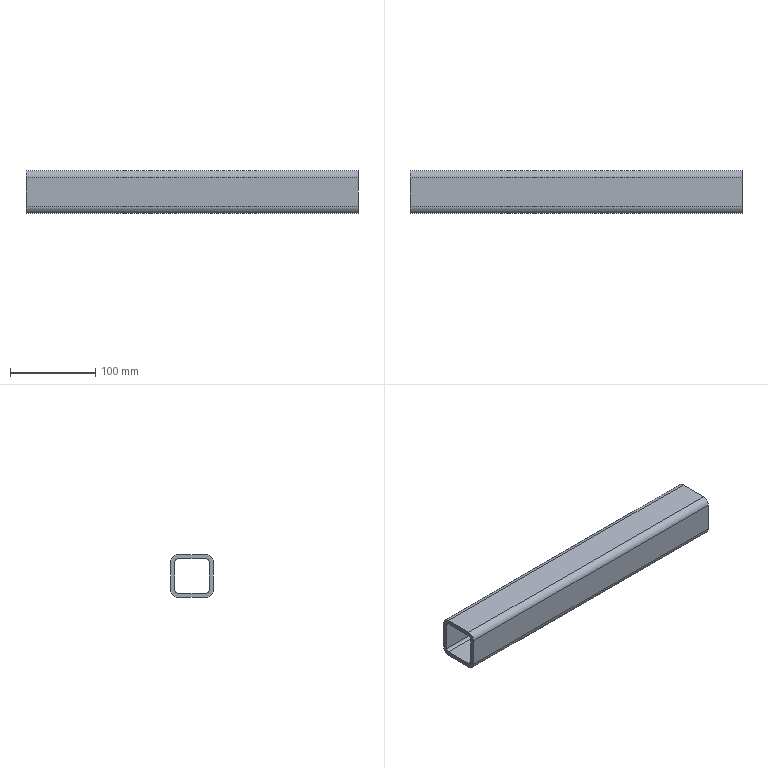Part | SolidWorks | features WeldMemberFeat 1, WeldmentFeature 1 | 1 solid | 18 faces | box 390 x 50 x 50 mm | volume 332587 mm3 | plane 10 | cylinder 8 | commonest cylinder face diameters 6 x4 16 x4
STEP:
#1=CARTESIAN_POINT('',(-88.434,25.,17.));
#2=VERTEX_POINT('',#1);
#3=CARTESIAN_POINT('',(-88.434,17.,25.));
#4=VERTEX_POINT('',#3);
#5=CARTESIAN_POINT('',(-88.434,17.,17.));
#6=DIRECTION('',(1.,0.,0.));
#7=DIRECTION('',(0.,0.,-1.));
#8=AXIS2_PLACEMENT_3D('',#5,#6,#7);
#9=CIRCLE('',#8,8.);
#10=EDGE_CURVE('',#2,#4,#9,.T.);
#11=ORIENTED_EDGE('',*,*,#10,.T.);
#12=CARTESIAN_POINT('',(301.566,17.,25.));
#13=VERTEX_POINT('',#12);
#14=CARTESIAN_POINT('',(301.566,17.,25.));
#15=DIRECTION('',(-1.,0.,0.));
#16=VECTOR('',#15,1000.);
#17=LINE('',#14,#16);
#18=EDGE_CURVE('',#13,#4,#17,.T.);
#19=ORIENTED_EDGE('',*,*,#18,.F.);
#20=CARTESIAN_POINT('',(301.566,25.,17.));
#21=VERTEX_POINT('',#20);
#22=CARTESIAN_POINT('',(301.566,17.,17.));
#23=DIRECTION('',(1.,0.,0.));
#24=DIRECTION('',(0.,0.,-1.));
#25=AXIS2_PLACEMENT_3D('',#22,#23,#24);
#26=CIRCLE('',#25,8.);
#27=EDGE_CURVE('',#21,#13,#26,.T.);
#28=ORIENTED_EDGE('',*,*,#27,.F.);
#29=CARTESIAN_POINT('',(301.566,25.,17.));
#30=DIRECTION('',(-1.,0.,0.));
#31=VECTOR('',#30,1000.);
#32=LINE('',#29,#31);
#33=EDGE_CURVE('',#21,#2,#32,.T.);
#34=ORIENTED_EDGE('',*,*,#33,.T.);
#35=EDGE_LOOP('',(#11,#19,#28,#34));
#36=FACE_OUTER_BOUND('',#35,.T.);
#37=CARTESIAN_POINT('',(301.566,17.,17.));
#38=DIRECTION('',(-1.,0.,0.));
#39=DIRECTION('',(0.,0.,1.));
#40=AXIS2_PLACEMENT_3D('',#37,#38,#39);
#41=CYLINDRICAL_SURFACE('',#40,8.);
#42=ADVANCED_FACE('',(#36),#41,.T.);
#43=CARTESIAN_POINT('',(-88.434,-17.,25.));
#44=VERTEX_POINT('',#43);
#45=CARTESIAN_POINT('',(-88.434,17.,25.));
#46=DIRECTION('',(0.,-1.,0.));
#47=VECTOR('',#46,1000.);
#48=LINE('',#45,#47);
#49=EDGE_CURVE('',#4,#44,#48,.T.);
#50=ORIENTED_EDGE('',*,*,#49,.T.);
#51=CARTESIAN_POINT('',(301.566,-17.,25.));
#52=VERTEX_POINT('',#51);
#53=CARTESIAN_POINT('',(301.566,-17.,25.));
#54=DIRECTION('',(-1.,0.,0.));
#55=VECTOR('',#54,1000.);
#56=LINE('',#53,#55);
#57=EDGE_CURVE('',#52,#44,#56,.T.);
#58=ORIENTED_EDGE('',*,*,#57,.F.);
#59=CARTESIAN_POINT('',(301.566,17.,25.));
#60=DIRECTION('',(0.,-1.,0.));
#61=VECTOR('',#60,1000.);
#62=LINE('',#59,#61);
#63=EDGE_CURVE('',#13,#52,#62,.T.);
#64=ORIENTED_EDGE('',*,*,#63,.F.);
#65=ORIENTED_EDGE('',*,*,#18,.T.);
#66=EDGE_LOOP('',(#50,#58,#64,#65));
#67=FACE_OUTER_BOUND('',#66,.T.);
#68=CARTESIAN_POINT('',(301.566,17.,25.));
#69=DIRECTION('',(0.,0.,-1.));
#70=DIRECTION('',(-1.,0.,0.));
#71=AXIS2_PLACEMENT_3D('',#68,#69,#70);
#72=PLANE('',#71);
#73=ADVANCED_FACE('',(#67),#72,.F.);
#74=CARTESIAN_POINT('',(-88.434,-25.,17.));
#75=VERTEX_POINT('',#74);
#76=CARTESIAN_POINT('',(-88.434,-17.,17.));
#77=DIRECTION('',(1.,0.,0.));
#78=DIRECTION('',(0.,0.,-1.));
#79=AXIS2_PLACEMENT_3D('',#76,#77,#78);
#80=CIRCLE('',#79,8.);
#81=EDGE_CURVE('',#44,#75,#80,.T.);
#82=ORIENTED_EDGE('',*,*,#81,.T.);
#83=CARTESIAN_POINT('',(301.566,-25.,17.));
#84=VERTEX_POINT('',#83);
#85=CARTESIAN_POINT('',(301.566,-25.,17.));
#86=DIRECTION('',(-1.,0.,0.));
#87=VECTOR('',#86,1000.);
#88=LINE('',#85,#87);
#89=EDGE_CURVE('',#84,#75,#88,.T.);
#90=ORIENTED_EDGE('',*,*,#89,.F.);
#91=CARTESIAN_POINT('',(301.566,-17.,17.));
#92=DIRECTION('',(1.,0.,0.));
#93=DIRECTION('',(0.,0.,-1.));
#94=AXIS2_PLACEMENT_3D('',#91,#92,#93);
#95=CIRCLE('',#94,8.);
#96=EDGE_CURVE('',#52,#84,#95,.T.);
#97=ORIENTED_EDGE('',*,*,#96,.F.);
#98=ORIENTED_EDGE('',*,*,#57,.T.);
#99=EDGE_LOOP('',(#82,#90,#97,#98));
#100=FACE_OUTER_BOUND('',#99,.T.);
#101=CARTESIAN_POINT('',(301.566,-17.,17.));
#102=DIRECTION('',(-1.,0.,0.));
#103=DIRECTION('',(0.,0.,1.));
#104=AXIS2_PLACEMENT_3D('',#101,#102,#103);
#105=CYLINDRICAL_SURFACE('',#104,8.);
#106=ADVANCED_FACE('',(#100),#105,.T.);
#107=CARTESIAN_POINT('',(-88.434,-25.,-17.));
#108=VERTEX_POINT('',#107);
#109=CARTESIAN_POINT('',(-88.434,-25.,-17.));
#110=DIRECTION('',(0.,0.,-1.));
#111=VECTOR('',#110,1000.);
#112=LINE('',#109,#111);
#113=EDGE_CURVE('',#75,#108,#112,.T.);
#114=ORIENTED_EDGE('',*,*,#113,.T.);
#115=CARTESIAN_POINT('',(301.566,-25.,-17.));
#116=VERTEX_POINT('',#115);
#117=CARTESIAN_POINT('',(301.566,-25.,-17.));
#118=DIRECTION('',(-1.,0.,0.));
#119=VECTOR('',#118,1000.);
#120=LINE('',#117,#119);
#121=EDGE_CURVE('',#116,#108,#120,.T.);
#122=ORIENTED_EDGE('',*,*,#121,.F.);
#123=CARTESIAN_POINT('',(301.566,-25.,-17.));
#124=DIRECTION('',(0.,0.,-1.));
#125=VECTOR('',#124,1000.);
#126=LINE('',#123,#125);
#127=EDGE_CURVE('',#84,#116,#126,.T.);
#128=ORIENTED_EDGE('',*,*,#127,.F.);
#129=ORIENTED_EDGE('',*,*,#89,.T.);
#130=EDGE_LOOP('',(#114,#122,#128,#129));
#131=FACE_OUTER_BOUND('',#130,.T.);
#132=CARTESIAN_POINT('',(301.566,-25.,-17.));
#133=DIRECTION('',(0.,1.,0.));
#134=DIRECTION('',(0.,0.,1.));
#135=AXIS2_PLACEMENT_3D('',#132,#133,#134);
#136=PLANE('',#135);
#137=ADVANCED_FACE('',(#131),#136,.F.);
#138=CARTESIAN_POINT('',(-88.434,-17.,-25.));
#139=VERTEX_POINT('',#138);
#140=CARTESIAN_POINT('',(-88.434,-17.,-17.));
#141=DIRECTION('',(1.,0.,0.));
#142=DIRECTION('',(0.,0.,-1.));
#143=AXIS2_PLACEMENT_3D('',#140,#141,#142);
#144=CIRCLE('',#143,8.);
#145=EDGE_CURVE('',#108,#139,#144,.T.);
#146=ORIENTED_EDGE('',*,*,#145,.T.);
#147=CARTESIAN_POINT('',(301.566,-17.,-25.));
#148=VERTEX_POINT('',#147);
#149=CARTESIAN_POINT('',(301.566,-17.,-25.));
#150=DIRECTION('',(-1.,0.,0.));
#151=VECTOR('',#150,1000.);
#152=LINE('',#149,#151);
#153=EDGE_CURVE('',#148,#139,#152,.T.);
#154=ORIENTED_EDGE('',*,*,#153,.F.);
#155=CARTESIAN_POINT('',(301.566,-17.,-17.));
#156=DIRECTION('',(1.,0.,0.));
#157=DIRECTION('',(0.,0.,-1.));
#158=AXIS2_PLACEMENT_3D('',#155,#156,#157);
#159=CIRCLE('',#158,8.);
#160=EDGE_CURVE('',#116,#148,#159,.T.);
#161=ORIENTED_EDGE('',*,*,#160,.F.);
#162=ORIENTED_EDGE('',*,*,#121,.T.);
#163=EDGE_LOOP('',(#146,#154,#161,#162));
#164=FACE_OUTER_BOUND('',#163,.T.);
#165=CARTESIAN_POINT('',(301.566,-17.,-17.));
#166=DIRECTION('',(-1.,0.,0.));
#167=DIRECTION('',(0.,0.,1.));
#168=AXIS2_PLACEMENT_3D('',#165,#166,#167);
#169=CYLINDRICAL_SURFACE('',#168,8.);
#170=ADVANCED_FACE('',(#164),#169,.T.);
#171=CARTESIAN_POINT('',(-88.434,17.,-25.));
#172=VERTEX_POINT('',#171);
#173=CARTESIAN_POINT('',(-88.434,-17.,-25.));
#174=DIRECTION('',(0.,1.,0.));
#175=VECTOR('',#174,1000.);
#176=LINE('',#173,#175);
#177=EDGE_CURVE('',#139,#172,#176,.T.);
#178=ORIENTED_EDGE('',*,*,#177,.T.);
#179=CARTESIAN_POINT('',(301.566,17.,-25.));
#180=VERTEX_POINT('',#179);
#181=CARTESIAN_POINT('',(301.566,17.,-25.));
#182=DIRECTION('',(-1.,0.,0.));
#183=VECTOR('',#182,1000.);
#184=LINE('',#181,#183);
#185=EDGE_CURVE('',#180,#172,#184,.T.);
#186=ORIENTED_EDGE('',*,*,#185,.F.);
#187=CARTESIAN_POINT('',(301.566,-17.,-25.));
#188=DIRECTION('',(0.,1.,0.));
#189=VECTOR('',#188,1000.);
#190=LINE('',#187,#189);
#191=EDGE_CURVE('',#148,#180,#190,.T.);
#192=ORIENTED_EDGE('',*,*,#191,.F.);
#193=ORIENTED_EDGE('',*,*,#153,.T.);
#194=EDGE_LOOP('',(#178,#186,#192,#193));
#195=FACE_OUTER_BOUND('',#194,.T.);
#196=CARTESIAN_POINT('',(301.566,-17.,-25.));
#197=DIRECTION('',(0.,0.,1.));
#198=DIRECTION('',(1.,0.,0.));
#199=AXIS2_PLACEMENT_3D('',#196,#197,#198);
#200=PLANE('',#199);
#201=ADVANCED_FACE('',(#195),#200,.F.);
#202=CARTESIAN_POINT('',(-88.434,25.,-17.));
#203=VERTEX_POINT('',#202);
#204=CARTESIAN_POINT('',(-88.434,17.,-17.));
#205=DIRECTION('',(1.,0.,0.));
#206=DIRECTION('',(0.,0.,-1.));
#207=AXIS2_PLACEMENT_3D('',#204,#205,#206);
#208=CIRCLE('',#207,8.);
#209=EDGE_CURVE('',#172,#203,#208,.T.);
#210=ORIENTED_EDGE('',*,*,#209,.T.);
#211=CARTESIAN_POINT('',(301.566,25.,-17.));
#212=VERTEX_POINT('',#211);
#213=CARTESIAN_POINT('',(301.566,25.,-17.));
#214=DIRECTION('',(-1.,0.,0.));
#215=VECTOR('',#214,1000.);
#216=LINE('',#213,#215);
#217=EDGE_CURVE('',#212,#203,#216,.T.);
#218=ORIENTED_EDGE('',*,*,#217,.F.);
#219=CARTESIAN_POINT('',(301.566,17.,-17.));
#220=DIRECTION('',(1.,0.,0.));
#221=DIRECTION('',(0.,0.,-1.));
#222=AXIS2_PLACEMENT_3D('',#219,#220,#221);
#223=CIRCLE('',#222,8.);
#224=EDGE_CURVE('',#180,#212,#223,.T.);
#225=ORIENTED_EDGE('',*,*,#224,.F.);
#226=ORIENTED_EDGE('',*,*,#185,.T.);
#227=EDGE_LOOP('',(#210,#218,#225,#226));
#228=FACE_OUTER_BOUND('',#227,.T.);
#229=CARTESIAN_POINT('',(301.566,17.,-17.));
#230=DIRECTION('',(-1.,0.,0.));
#231=DIRECTION('',(0.,0.,1.));
#232=AXIS2_PLACEMENT_3D('',#229,#230,#231);
#233=CYLINDRICAL_SURFACE('',#232,8.);
#234=ADVANCED_FACE('',(#228),#233,.T.);
#235=CARTESIAN_POINT('',(-88.434,-17.,20.));
#236=VERTEX_POINT('',#235);
#237=CARTESIAN_POINT('',(-88.434,-20.,17.));
#238=VERTEX_POINT('',#237);
#239=CARTESIAN_POINT('',(-88.434,-17.,17.));
#240=DIRECTION('',(1.,0.,0.));
#241=DIRECTION('',(0.,0.,-1.));
#242=AXIS2_PLACEMENT_3D('',#239,#240,#241);
#243=CIRCLE('',#242,3.);
#244=EDGE_CURVE('',#236,#238,#243,.T.);
#245=ORIENTED_EDGE('',*,*,#244,.F.);
#246=CARTESIAN_POINT('',(301.566,-17.,20.));
#247=VERTEX_POINT('',#246);
#248=CARTESIAN_POINT('',(301.566,-17.,20.));
#249=DIRECTION('',(-1.,0.,0.));
#250=VECTOR('',#249,1000.);
#251=LINE('',#248,#250);
#252=EDGE_CURVE('',#247,#236,#251,.T.);
#253=ORIENTED_EDGE('',*,*,#252,.F.);
#254=CARTESIAN_POINT('',(301.566,-20.,17.));
#255=VERTEX_POINT('',#254);
#256=CARTESIAN_POINT('',(301.566,-17.,17.));
#257=DIRECTION('',(1.,0.,0.));
#258=DIRECTION('',(0.,0.,-1.));
#259=AXIS2_PLACEMENT_3D('',#256,#257,#258);
#260=CIRCLE('',#259,3.);
#261=EDGE_CURVE('',#247,#255,#260,.T.);
#262=ORIENTED_EDGE('',*,*,#261,.T.);
#263=CARTESIAN_POINT('',(301.566,-20.,17.));
#264=DIRECTION('',(-1.,0.,0.));
#265=VECTOR('',#264,1000.);
#266=LINE('',#263,#265);
#267=EDGE_CURVE('',#255,#238,#266,.T.);
#268=ORIENTED_EDGE('',*,*,#267,.T.);
#269=EDGE_LOOP('',(#245,#253,#262,#268));
#270=FACE_OUTER_BOUND('',#269,.T.);
#271=CARTESIAN_POINT('',(301.566,-17.,17.));
#272=DIRECTION('',(-1.,0.,0.));
#273=DIRECTION('',(0.,0.,1.));
#274=AXIS2_PLACEMENT_3D('',#271,#272,#273);
#275=CYLINDRICAL_SURFACE('',#274,3.);
#276=ADVANCED_FACE('',(#270),#275,.F.);
#277=CARTESIAN_POINT('',(-88.434,17.,20.));
#278=VERTEX_POINT('',#277);
#279=CARTESIAN_POINT('',(-88.434,17.,20.));
#280=DIRECTION('',(0.,-1.,0.));
#281=VECTOR('',#280,1000.);
#282=LINE('',#279,#281);
#283=EDGE_CURVE('',#278,#236,#282,.T.);
#284=ORIENTED_EDGE('',*,*,#283,.F.);
#285=CARTESIAN_POINT('',(301.566,17.,20.));
#286=VERTEX_POINT('',#285);
#287=CARTESIAN_POINT('',(301.566,17.,20.));
#288=DIRECTION('',(-1.,0.,0.));
#289=VECTOR('',#288,1000.);
#290=LINE('',#287,#289);
#291=EDGE_CURVE('',#286,#278,#290,.T.);
#292=ORIENTED_EDGE('',*,*,#291,.F.);
#293=CARTESIAN_POINT('',(301.566,17.,20.));
#294=DIRECTION('',(0.,-1.,0.));
#295=VECTOR('',#294,1000.);
#296=LINE('',#293,#295);
#297=EDGE_CURVE('',#286,#247,#296,.T.);
#298=ORIENTED_EDGE('',*,*,#297,.T.);
#299=ORIENTED_EDGE('',*,*,#252,.T.);
#300=EDGE_LOOP('',(#284,#292,#298,#299));
#301=FACE_OUTER_BOUND('',#300,.T.);
#302=CARTESIAN_POINT('',(301.566,17.,20.));
#303=DIRECTION('',(0.,0.,-1.));
#304=DIRECTION('',(-1.,0.,0.));
#305=AXIS2_PLACEMENT_3D('',#302,#303,#304);
#306=PLANE('',#305);
#307=ADVANCED_FACE('',(#301),#306,.T.);
#308=CARTESIAN_POINT('',(-88.434,20.,17.));
#309=VERTEX_POINT('',#308);
#310=CARTESIAN_POINT('',(-88.434,17.,17.));
#311=DIRECTION('',(1.,0.,0.));
#312=DIRECTION('',(0.,0.,-1.));
#313=AXIS2_PLACEMENT_3D('',#310,#311,#312);
#314=CIRCLE('',#313,3.);
#315=EDGE_CURVE('',#309,#278,#314,.T.);
#316=ORIENTED_EDGE('',*,*,#315,.F.);
#317=CARTESIAN_POINT('',(301.566,20.,17.));
#318=VERTEX_POINT('',#317);
#319=CARTESIAN_POINT('',(301.566,20.,17.));
#320=DIRECTION('',(-1.,0.,0.));
#321=VECTOR('',#320,1000.);
#322=LINE('',#319,#321);
#323=EDGE_CURVE('',#318,#309,#322,.T.);
#324=ORIENTED_EDGE('',*,*,#323,.F.);
#325=CARTESIAN_POINT('',(301.566,17.,17.));
#326=DIRECTION('',(1.,0.,0.));
#327=DIRECTION('',(0.,0.,-1.));
#328=AXIS2_PLACEMENT_3D('',#325,#326,#327);
#329=CIRCLE('',#328,3.);
#330=EDGE_CURVE('',#318,#286,#329,.T.);
#331=ORIENTED_EDGE('',*,*,#330,.T.);
#332=ORIENTED_EDGE('',*,*,#291,.T.);
#333=EDGE_LOOP('',(#316,#324,#331,#332));
#334=FACE_OUTER_BOUND('',#333,.T.);
#335=CARTESIAN_POINT('',(301.566,17.,17.));
#336=DIRECTION('',(-1.,0.,0.));
#337=DIRECTION('',(0.,0.,1.));
#338=AXIS2_PLACEMENT_3D('',#335,#336,#337);
#339=CYLINDRICAL_SURFACE('',#338,3.);
#340=ADVANCED_FACE('',(#334),#339,.F.);
#341=CARTESIAN_POINT('',(-88.434,20.,-17.));
#342=VERTEX_POINT('',#341);
#343=CARTESIAN_POINT('',(-88.434,20.,17.));
#344=DIRECTION('',(0.,0.,1.));
#345=VECTOR('',#344,1000.);
#346=LINE('',#343,#345);
#347=EDGE_CURVE('',#342,#309,#346,.T.);
#348=ORIENTED_EDGE('',*,*,#347,.F.);
#349=CARTESIAN_POINT('',(301.566,20.,-17.));
#350=VERTEX_POINT('',#349);
#351=CARTESIAN_POINT('',(301.566,20.,-17.));
#352=DIRECTION('',(-1.,0.,0.));
#353=VECTOR('',#352,1000.);
#354=LINE('',#351,#353);
#355=EDGE_CURVE('',#350,#342,#354,.T.);
#356=ORIENTED_EDGE('',*,*,#355,.F.);
#357=CARTESIAN_POINT('',(301.566,20.,17.));
#358=DIRECTION('',(0.,0.,1.));
#359=VECTOR('',#358,1000.);
#360=LINE('',#357,#359);
#361=EDGE_CURVE('',#350,#318,#360,.T.);
#362=ORIENTED_EDGE('',*,*,#361,.T.);
#363=ORIENTED_EDGE('',*,*,#323,.T.);
#364=EDGE_LOOP('',(#348,#356,#362,#363));
#365=FACE_OUTER_BOUND('',#364,.T.);
#366=CARTESIAN_POINT('',(301.566,20.,17.));
#367=DIRECTION('',(0.,-1.,0.));
#368=DIRECTION('',(0.,0.,-1.));
#369=AXIS2_PLACEMENT_3D('',#366,#367,#368);
#370=PLANE('',#369);
#371=ADVANCED_FACE('',(#365),#370,.T.);
#372=CARTESIAN_POINT('',(-88.434,17.,-20.));
#373=VERTEX_POINT('',#372);
#374=CARTESIAN_POINT('',(-88.434,17.,-17.));
#375=DIRECTION('',(1.,0.,0.));
#376=DIRECTION('',(0.,0.,-1.));
#377=AXIS2_PLACEMENT_3D('',#374,#375,#376);
#378=CIRCLE('',#377,3.);
#379=EDGE_CURVE('',#373,#342,#378,.T.);
#380=ORIENTED_EDGE('',*,*,#379,.F.);
#381=CARTESIAN_POINT('',(301.566,17.,-20.));
#382=VERTEX_POINT('',#381);
#383=CARTESIAN_POINT('',(301.566,17.,-20.));
#384=DIRECTION('',(-1.,0.,0.));
#385=VECTOR('',#384,1000.);
#386=LINE('',#383,#385);
#387=EDGE_CURVE('',#382,#373,#386,.T.);
#388=ORIENTED_EDGE('',*,*,#387,.F.);
#389=CARTESIAN_POINT('',(301.566,17.,-17.));
#390=DIRECTION('',(1.,0.,0.));
#391=DIRECTION('',(0.,0.,-1.));
#392=AXIS2_PLACEMENT_3D('',#389,#390,#391);
#393=CIRCLE('',#392,3.);
#394=EDGE_CURVE('',#382,#350,#393,.T.);
#395=ORIENTED_EDGE('',*,*,#394,.T.);
#396=ORIENTED_EDGE('',*,*,#355,.T.);
#397=EDGE_LOOP('',(#380,#388,#395,#396));
#398=FACE_OUTER_BOUND('',#397,.T.);
#399=CARTESIAN_POINT('',(301.566,17.,-17.));
#400=DIRECTION('',(-1.,0.,0.));
#401=DIRECTION('',(0.,0.,1.));
#402=AXIS2_PLACEMENT_3D('',#399,#400,#401);
#403=CYLINDRICAL_SURFACE('',#402,3.);
#404=ADVANCED_FACE('',(#398),#403,.F.);
#405=CARTESIAN_POINT('',(-88.434,-17.,-20.));
#406=VERTEX_POINT('',#405);
#407=CARTESIAN_POINT('',(-88.434,-17.,-20.));
#408=DIRECTION('',(0.,1.,0.));
#409=VECTOR('',#408,1000.);
#410=LINE('',#407,#409);
#411=EDGE_CURVE('',#406,#373,#410,.T.);
#412=ORIENTED_EDGE('',*,*,#411,.F.);
#413=CARTESIAN_POINT('',(301.566,-17.,-20.));
#414=VERTEX_POINT('',#413);
#415=CARTESIAN_POINT('',(301.566,-17.,-20.));
#416=DIRECTION('',(-1.,0.,0.));
#417=VECTOR('',#416,1000.);
#418=LINE('',#415,#417);
#419=EDGE_CURVE('',#414,#406,#418,.T.);
#420=ORIENTED_EDGE('',*,*,#419,.F.);
#421=CARTESIAN_POINT('',(301.566,-17.,-20.));
#422=DIRECTION('',(0.,1.,0.));
#423=VECTOR('',#422,1000.);
#424=LINE('',#421,#423);
#425=EDGE_CURVE('',#414,#382,#424,.T.);
#426=ORIENTED_EDGE('',*,*,#425,.T.);
#427=ORIENTED_EDGE('',*,*,#387,.T.);
#428=EDGE_LOOP('',(#412,#420,#426,#427));
#429=FACE_OUTER_BOUND('',#428,.T.);
#430=CARTESIAN_POINT('',(301.566,-17.,-20.));
#431=DIRECTION('',(0.,0.,1.));
#432=DIRECTION('',(1.,0.,0.));
#433=AXIS2_PLACEMENT_3D('',#430,#431,#432);
#434=PLANE('',#433);
#435=ADVANCED_FACE('',(#429),#434,.T.);
#436=CARTESIAN_POINT('',(-88.434,-20.,-17.));
#437=VERTEX_POINT('',#436);
#438=CARTESIAN_POINT('',(-88.434,-17.,-17.));
#439=DIRECTION('',(1.,0.,0.));
#440=DIRECTION('',(0.,0.,-1.));
#441=AXIS2_PLACEMENT_3D('',#438,#439,#440);
#442=CIRCLE('',#441,3.);
#443=EDGE_CURVE('',#437,#406,#442,.T.);
#444=ORIENTED_EDGE('',*,*,#443,.F.);
#445=CARTESIAN_POINT('',(301.566,-20.,-17.));
#446=VERTEX_POINT('',#445);
#447=CARTESIAN_POINT('',(301.566,-20.,-17.));
#448=DIRECTION('',(-1.,0.,0.));
#449=VECTOR('',#448,1000.);
#450=LINE('',#447,#449);
#451=EDGE_CURVE('',#446,#437,#450,.T.);
#452=ORIENTED_EDGE('',*,*,#451,.F.);
#453=CARTESIAN_POINT('',(301.566,-17.,-17.));
#454=DIRECTION('',(1.,0.,0.));
#455=DIRECTION('',(0.,0.,-1.));
#456=AXIS2_PLACEMENT_3D('',#453,#454,#455);
#457=CIRCLE('',#456,3.);
#458=EDGE_CURVE('',#446,#414,#457,.T.);
#459=ORIENTED_EDGE('',*,*,#458,.T.);
#460=ORIENTED_EDGE('',*,*,#419,.T.);
#461=EDGE_LOOP('',(#444,#452,#459,#460));
#462=FACE_OUTER_BOUND('',#461,.T.);
#463=CARTESIAN_POINT('',(301.566,-17.,-17.));
#464=DIRECTION('',(-1.,0.,0.));
#465=DIRECTION('',(0.,0.,1.));
#466=AXIS2_PLACEMENT_3D('',#463,#464,#465);
#467=CYLINDRICAL_SURFACE('',#466,3.);
#468=ADVANCED_FACE('',(#462),#467,.F.);
#469=CARTESIAN_POINT('',(-88.434,-20.,-17.));
#470=DIRECTION('',(0.,0.,-1.));
#471=VECTOR('',#470,1000.);
#472=LINE('',#469,#471);
#473=EDGE_CURVE('',#238,#437,#472,.T.);
#474=ORIENTED_EDGE('',*,*,#473,.F.);
#475=ORIENTED_EDGE('',*,*,#267,.F.);
#476=CARTESIAN_POINT('',(301.566,-20.,-17.));
#477=DIRECTION('',(0.,0.,-1.));
#478=VECTOR('',#477,1000.);
#479=LINE('',#476,#478);
#480=EDGE_CURVE('',#255,#446,#479,.T.);
#481=ORIENTED_EDGE('',*,*,#480,.T.);
#482=ORIENTED_EDGE('',*,*,#451,.T.);
#483=EDGE_LOOP('',(#474,#475,#481,#482));
#484=FACE_OUTER_BOUND('',#483,.T.);
#485=CARTESIAN_POINT('',(301.566,-20.,-17.));
#486=DIRECTION('',(0.,1.,0.));
#487=DIRECTION('',(0.,0.,1.));
#488=AXIS2_PLACEMENT_3D('',#485,#486,#487);
#489=PLANE('',#488);
#490=ADVANCED_FACE('',(#484),#489,.T.);
#491=CARTESIAN_POINT('',(-88.434,25.,17.));
#492=DIRECTION('',(0.,0.,1.));
#493=VECTOR('',#492,1000.);
#494=LINE('',#491,#493);
#495=EDGE_CURVE('',#203,#2,#494,.T.);
#496=ORIENTED_EDGE('',*,*,#495,.T.);
#497=ORIENTED_EDGE('',*,*,#33,.F.);
#498=CARTESIAN_POINT('',(301.566,25.,17.));
#499=DIRECTION('',(0.,0.,1.));
#500=VECTOR('',#499,1000.);
#501=LINE('',#498,#500);
#502=EDGE_CURVE('',#212,#21,#501,.T.);
#503=ORIENTED_EDGE('',*,*,#502,.F.);
#504=ORIENTED_EDGE('',*,*,#217,.T.);
#505=EDGE_LOOP('',(#496,#497,#503,#504));
#506=FACE_OUTER_BOUND('',#505,.T.);
#507=CARTESIAN_POINT('',(301.566,25.,17.));
#508=DIRECTION('',(0.,-1.,0.));
#509=DIRECTION('',(0.,0.,-1.));
#510=AXIS2_PLACEMENT_3D('',#507,#508,#509);
#511=PLANE('',#510);
#512=ADVANCED_FACE('',(#506),#511,.F.);
#513=ORIENTED_EDGE('',*,*,#261,.F.);
#514=ORIENTED_EDGE('',*,*,#297,.F.);
#515=ORIENTED_EDGE('',*,*,#330,.F.);
#516=ORIENTED_EDGE('',*,*,#361,.F.);
#517=ORIENTED_EDGE('',*,*,#394,.F.);
#518=ORIENTED_EDGE('',*,*,#425,.F.);
#519=ORIENTED_EDGE('',*,*,#458,.F.);
#520=ORIENTED_EDGE('',*,*,#480,.F.);
#521=EDGE_LOOP('',(#513,#514,#515,#516,#517,#518,#519,#520));
#522=FACE_BOUND('',#521,.T.);
#523=ORIENTED_EDGE('',*,*,#27,.T.);
#524=ORIENTED_EDGE('',*,*,#63,.T.);
#525=ORIENTED_EDGE('',*,*,#96,.T.);
#526=ORIENTED_EDGE('',*,*,#127,.T.);
#527=ORIENTED_EDGE('',*,*,#160,.T.);
#528=ORIENTED_EDGE('',*,*,#191,.T.);
#529=ORIENTED_EDGE('',*,*,#224,.T.);
#530=ORIENTED_EDGE('',*,*,#502,.T.);
#531=EDGE_LOOP('',(#523,#524,#525,#526,#527,#528,#529,#530));
#532=FACE_OUTER_BOUND('',#531,.T.);
#533=CARTESIAN_POINT('',(301.566,17.,17.));
#534=DIRECTION('',(1.,0.,0.));
#535=DIRECTION('',(0.,0.,-1.));
#536=AXIS2_PLACEMENT_3D('',#533,#534,#535);
#537=PLANE('',#536);
#538=ADVANCED_FACE('',(#522,#532),#537,.T.);
#539=ORIENTED_EDGE('',*,*,#244,.T.);
#540=ORIENTED_EDGE('',*,*,#473,.T.);
#541=ORIENTED_EDGE('',*,*,#443,.T.);
#542=ORIENTED_EDGE('',*,*,#411,.T.);
#543=ORIENTED_EDGE('',*,*,#379,.T.);
#544=ORIENTED_EDGE('',*,*,#347,.T.);
#545=ORIENTED_EDGE('',*,*,#315,.T.);
#546=ORIENTED_EDGE('',*,*,#283,.T.);
#547=EDGE_LOOP('',(#539,#540,#541,#542,#543,#544,#545,#546));
#548=FACE_BOUND('',#547,.T.);
#549=ORIENTED_EDGE('',*,*,#10,.F.);
#550=ORIENTED_EDGE('',*,*,#495,.F.);
#551=ORIENTED_EDGE('',*,*,#209,.F.);
#552=ORIENTED_EDGE('',*,*,#177,.F.);
#553=ORIENTED_EDGE('',*,*,#145,.F.);
#554=ORIENTED_EDGE('',*,*,#113,.F.);
#555=ORIENTED_EDGE('',*,*,#81,.F.);
#556=ORIENTED_EDGE('',*,*,#49,.F.);
#557=EDGE_LOOP('',(#549,#550,#551,#552,#553,#554,#555,#556));
#558=FACE_OUTER_BOUND('',#557,.T.);
#559=CARTESIAN_POINT('',(-88.434,17.,17.));
#560=DIRECTION('',(1.,0.,0.));
#561=DIRECTION('',(0.,0.,-1.));
#562=AXIS2_PLACEMENT_3D('',#559,#560,#561);
#563=PLANE('',#562);
#564=ADVANCED_FACE('',(#548,#558),#563,.F.);
#565=CLOSED_SHELL('',(#42,#73,#106,#137,#170,#201,#234,#276,#307,#340,#371,#404,#435,#468,#490,#512,#538,#564));
#566=MANIFOLD_SOLID_BREP('',#565);
#567=CARTESIAN_POINT('',(0.,0.,0.));
#568=DIRECTION('',(0.,0.,1.));
#569=DIRECTION('',(1.,0.,0.));
#570=AXIS2_PLACEMENT_3D('',#567,#568,#569);
#571=(LENGTH_UNIT()NAMED_UNIT(*)SI_UNIT(.MILLI.,.METRE.));
#572=UNCERTAINTY_MEASURE_WITH_UNIT(LENGTH_MEASURE(0.00001),#571,'','');
#573=(NAMED_UNIT(*)PLANE_ANGLE_UNIT()SI_UNIT($,.RADIAN.));
#574=(NAMED_UNIT(*)SI_UNIT($,.STERADIAN.)SOLID_ANGLE_UNIT());
#575=(GEOMETRIC_REPRESENTATION_CONTEXT(3)GLOBAL_UNCERTAINTY_ASSIGNED_CONTEXT((#572))GLOBAL_UNIT_ASSIGNED_CONTEXT((#571,#573,#574))REPRESENTATION_CONTEXT('',''));
#576=ADVANCED_BREP_SHAPE_REPRESENTATION('',(#566,#570),#575);